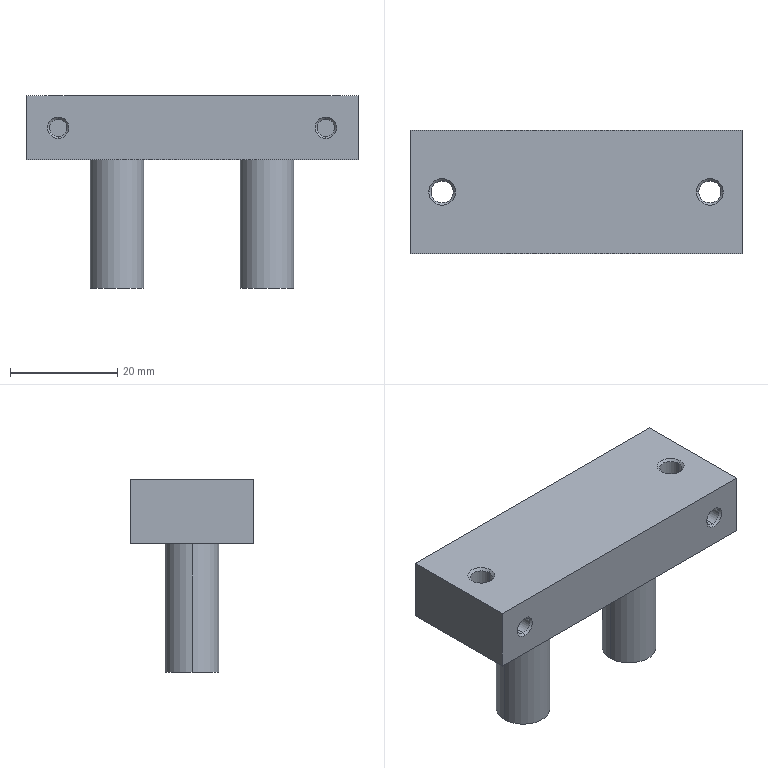Part | STEP file | B_CXSM20-10-Z73 | 1 solid | 40 faces | box 62 x 23 x 36 mm | volume 20357 mm3 | cylinder 16 | cone 12 | plane 12 | commonest cylinder face diameters 3.24 x8 4.13 x4 10 x4
STEP:
#1=CARTESIAN_POINT('',(22.935,12.5,23.565));
#2=VERTEX_POINT('',#1);
#3=CARTESIAN_POINT('',(27.065,12.5,23.565));
#4=VERTEX_POINT('',#3);
#5=CARTESIAN_POINT('',(25.,12.5,23.565));
#6=DIRECTION('',(0.,0.,1.));
#7=DIRECTION('',(1.,0.,0.));
#8=AXIS2_PLACEMENT_3D('',#5,#6,#7);
#9=CIRCLE('',#8,2.065);
#10=EDGE_CURVE('',#2,#4,#9,.T.);
#11=ORIENTED_EDGE('',*,*,#10,.F.);
#12=CARTESIAN_POINT('',(22.5,12.5,24.));
#13=VERTEX_POINT('',#12);
#14=CARTESIAN_POINT('',(22.5,12.5,24.));
#15=DIRECTION('',(-0.7071,0.,0.7071));
#16=VECTOR('',#15,1000.);
#17=LINE('',#14,#16);
#18=EDGE_CURVE('',#2,#13,#17,.T.);
#19=ORIENTED_EDGE('',*,*,#18,.T.);
#20=CARTESIAN_POINT('',(27.5,12.5,24.));
#21=VERTEX_POINT('',#20);
#22=CARTESIAN_POINT('',(25.,12.5,24.));
#23=DIRECTION('',(0.,0.,-1.));
#24=DIRECTION('',(1.,0.,0.));
#25=AXIS2_PLACEMENT_3D('',#22,#23,#24);
#26=CIRCLE('',#25,2.5);
#27=EDGE_CURVE('',#21,#13,#26,.T.);
#28=ORIENTED_EDGE('',*,*,#27,.F.);
#29=CARTESIAN_POINT('',(27.5,12.5,24.));
#30=DIRECTION('',(0.7071,0.,0.7071));
#31=VECTOR('',#30,1000.);
#32=LINE('',#29,#31);
#33=EDGE_CURVE('',#4,#21,#32,.T.);
#34=ORIENTED_EDGE('',*,*,#33,.F.);
#35=EDGE_LOOP('',(#11,#19,#28,#34));
#36=FACE_OUTER_BOUND('',#35,.T.);
#37=CARTESIAN_POINT('',(25.,12.5,24.));
#38=DIRECTION('',(0.,0.,1.));
#39=DIRECTION('',(1.,0.,0.));
#40=AXIS2_PLACEMENT_3D('',#37,#38,#39);
#41=CONICAL_SURFACE('',#40,2.5,0.7854);
#42=ADVANCED_FACE('',(#36),#41,.F.);
#43=CARTESIAN_POINT('',(-27.065,12.5,23.565));
#44=VERTEX_POINT('',#43);
#45=CARTESIAN_POINT('',(-22.935,12.5,23.565));
#46=VERTEX_POINT('',#45);
#47=CARTESIAN_POINT('',(-25.,12.5,23.565));
#48=DIRECTION('',(0.,0.,1.));
#49=DIRECTION('',(1.,0.,0.));
#50=AXIS2_PLACEMENT_3D('',#47,#48,#49);
#51=CIRCLE('',#50,2.065);
#52=EDGE_CURVE('',#44,#46,#51,.T.);
#53=ORIENTED_EDGE('',*,*,#52,.F.);
#54=CARTESIAN_POINT('',(-27.5,12.5,24.));
#55=VERTEX_POINT('',#54);
#56=CARTESIAN_POINT('',(-27.5,12.5,24.));
#57=DIRECTION('',(-0.7071,0.,0.7071));
#58=VECTOR('',#57,1000.);
#59=LINE('',#56,#58);
#60=EDGE_CURVE('',#44,#55,#59,.T.);
#61=ORIENTED_EDGE('',*,*,#60,.T.);
#62=CARTESIAN_POINT('',(-22.5,12.5,24.));
#63=VERTEX_POINT('',#62);
#64=CARTESIAN_POINT('',(-25.,12.5,24.));
#65=DIRECTION('',(0.,0.,-1.));
#66=DIRECTION('',(1.,0.,0.));
#67=AXIS2_PLACEMENT_3D('',#64,#65,#66);
#68=CIRCLE('',#67,2.5);
#69=EDGE_CURVE('',#63,#55,#68,.T.);
#70=ORIENTED_EDGE('',*,*,#69,.F.);
#71=CARTESIAN_POINT('',(-22.5,12.5,24.));
#72=DIRECTION('',(0.7071,0.,0.7071));
#73=VECTOR('',#72,1000.);
#74=LINE('',#71,#73);
#75=EDGE_CURVE('',#46,#63,#74,.T.);
#76=ORIENTED_EDGE('',*,*,#75,.F.);
#77=EDGE_LOOP('',(#53,#61,#70,#76));
#78=FACE_OUTER_BOUND('',#77,.T.);
#79=CARTESIAN_POINT('',(-25.,12.5,24.));
#80=DIRECTION('',(0.,0.,1.));
#81=DIRECTION('',(1.,0.,0.));
#82=AXIS2_PLACEMENT_3D('',#79,#80,#81);
#83=CONICAL_SURFACE('',#82,2.5,0.7854);
#84=ADVANCED_FACE('',(#78),#83,.F.);
#85=CARTESIAN_POINT('',(-25.,23.62,16.38));
#86=VERTEX_POINT('',#85);
#87=CARTESIAN_POINT('',(-25.,23.62,19.62));
#88=VERTEX_POINT('',#87);
#89=CARTESIAN_POINT('',(-25.,23.62,18.));
#90=DIRECTION('',(0.,1.,0.));
#91=DIRECTION('',(-1.,0.,0.));
#92=AXIS2_PLACEMENT_3D('',#89,#90,#91);
#93=CIRCLE('',#92,1.62);
#94=EDGE_CURVE('',#86,#88,#93,.T.);
#95=ORIENTED_EDGE('',*,*,#94,.F.);
#96=CARTESIAN_POINT('',(-25.,24.,16.));
#97=VERTEX_POINT('',#96);
#98=CARTESIAN_POINT('',(-25.,24.,16.));
#99=DIRECTION('',(0.,0.7071,-0.7071));
#100=VECTOR('',#99,1000.);
#101=LINE('',#98,#100);
#102=EDGE_CURVE('',#86,#97,#101,.T.);
#103=ORIENTED_EDGE('',*,*,#102,.T.);
#104=CARTESIAN_POINT('',(-25.,24.,20.));
#105=VERTEX_POINT('',#104);
#106=CARTESIAN_POINT('',(-25.,24.,18.));
#107=DIRECTION('',(0.,-1.,0.));
#108=DIRECTION('',(0.,0.,1.));
#109=AXIS2_PLACEMENT_3D('',#106,#107,#108);
#110=CIRCLE('',#109,2.);
#111=EDGE_CURVE('',#105,#97,#110,.T.);
#112=ORIENTED_EDGE('',*,*,#111,.F.);
#113=CARTESIAN_POINT('',(-25.,24.,20.));
#114=DIRECTION('',(0.,0.7071,0.7071));
#115=VECTOR('',#114,1000.);
#116=LINE('',#113,#115);
#117=EDGE_CURVE('',#88,#105,#116,.T.);
#118=ORIENTED_EDGE('',*,*,#117,.F.);
#119=EDGE_LOOP('',(#95,#103,#112,#118));
#120=FACE_OUTER_BOUND('',#119,.T.);
#121=CARTESIAN_POINT('',(-25.,24.,18.));
#122=DIRECTION('',(0.,1.,0.));
#123=DIRECTION('',(0.,0.,1.));
#124=AXIS2_PLACEMENT_3D('',#121,#122,#123);
#125=CONICAL_SURFACE('',#124,2.,0.7854);
#126=ADVANCED_FACE('',(#120),#125,.F.);
#127=CARTESIAN_POINT('',(25.,23.62,16.38));
#128=VERTEX_POINT('',#127);
#129=CARTESIAN_POINT('',(25.,23.62,19.62));
#130=VERTEX_POINT('',#129);
#131=CARTESIAN_POINT('',(25.,23.62,18.));
#132=DIRECTION('',(0.,1.,0.));
#133=DIRECTION('',(-1.,0.,0.));
#134=AXIS2_PLACEMENT_3D('',#131,#132,#133);
#135=CIRCLE('',#134,1.62);
#136=EDGE_CURVE('',#128,#130,#135,.T.);
#137=ORIENTED_EDGE('',*,*,#136,.F.);
#138=CARTESIAN_POINT('',(25.,24.,16.));
#139=VERTEX_POINT('',#138);
#140=CARTESIAN_POINT('',(25.,24.,16.));
#141=DIRECTION('',(0.,0.7071,-0.7071));
#142=VECTOR('',#141,1000.);
#143=LINE('',#140,#142);
#144=EDGE_CURVE('',#128,#139,#143,.T.);
#145=ORIENTED_EDGE('',*,*,#144,.T.);
#146=CARTESIAN_POINT('',(25.,24.,20.));
#147=VERTEX_POINT('',#146);
#148=CARTESIAN_POINT('',(25.,24.,18.));
#149=DIRECTION('',(0.,-1.,0.));
#150=DIRECTION('',(0.,0.,1.));
#151=AXIS2_PLACEMENT_3D('',#148,#149,#150);
#152=CIRCLE('',#151,2.);
#153=EDGE_CURVE('',#147,#139,#152,.T.);
#154=ORIENTED_EDGE('',*,*,#153,.F.);
#155=CARTESIAN_POINT('',(25.,24.,20.));
#156=DIRECTION('',(0.,0.7071,0.7071));
#157=VECTOR('',#156,1000.);
#158=LINE('',#155,#157);
#159=EDGE_CURVE('',#130,#147,#158,.T.);
#160=ORIENTED_EDGE('',*,*,#159,.F.);
#161=EDGE_LOOP('',(#137,#145,#154,#160));
#162=FACE_OUTER_BOUND('',#161,.T.);
#163=CARTESIAN_POINT('',(25.,24.,18.));
#164=DIRECTION('',(0.,1.,0.));
#165=DIRECTION('',(0.,0.,1.));
#166=AXIS2_PLACEMENT_3D('',#163,#164,#165);
#167=CONICAL_SURFACE('',#166,2.,0.7854);
#168=ADVANCED_FACE('',(#162),#167,.F.);
#169=CARTESIAN_POINT('',(25.,1.38,19.62));
#170=VERTEX_POINT('',#169);
#171=CARTESIAN_POINT('',(25.,1.38,16.38));
#172=VERTEX_POINT('',#171);
#173=CARTESIAN_POINT('',(25.,1.38,18.));
#174=DIRECTION('',(0.,-1.,0.));
#175=DIRECTION('',(1.,0.,0.));
#176=AXIS2_PLACEMENT_3D('',#173,#174,#175);
#177=CIRCLE('',#176,1.62);
#178=EDGE_CURVE('',#170,#172,#177,.T.);
#179=ORIENTED_EDGE('',*,*,#178,.F.);
#180=CARTESIAN_POINT('',(25.,1.,20.));
#181=VERTEX_POINT('',#180);
#182=CARTESIAN_POINT('',(25.,1.,20.));
#183=DIRECTION('',(0.,-0.7071,0.7071));
#184=VECTOR('',#183,1000.);
#185=LINE('',#182,#184);
#186=EDGE_CURVE('',#170,#181,#185,.T.);
#187=ORIENTED_EDGE('',*,*,#186,.T.);
#188=CARTESIAN_POINT('',(25.,1.,16.));
#189=VERTEX_POINT('',#188);
#190=CARTESIAN_POINT('',(25.,1.,18.));
#191=DIRECTION('',(0.,1.,0.));
#192=DIRECTION('',(0.,0.,-1.));
#193=AXIS2_PLACEMENT_3D('',#190,#191,#192);
#194=CIRCLE('',#193,2.);
#195=EDGE_CURVE('',#189,#181,#194,.T.);
#196=ORIENTED_EDGE('',*,*,#195,.F.);
#197=CARTESIAN_POINT('',(25.,1.,16.));
#198=DIRECTION('',(0.,-0.7071,-0.7071));
#199=VECTOR('',#198,1000.);
#200=LINE('',#197,#199);
#201=EDGE_CURVE('',#172,#189,#200,.T.);
#202=ORIENTED_EDGE('',*,*,#201,.F.);
#203=EDGE_LOOP('',(#179,#187,#196,#202));
#204=FACE_OUTER_BOUND('',#203,.T.);
#205=CARTESIAN_POINT('',(25.,1.,18.));
#206=DIRECTION('',(0.,-1.,0.));
#207=DIRECTION('',(0.,0.,-1.));
#208=AXIS2_PLACEMENT_3D('',#205,#206,#207);
#209=CONICAL_SURFACE('',#208,2.,0.7854);
#210=ADVANCED_FACE('',(#204),#209,.F.);
#211=CARTESIAN_POINT('',(-25.,1.38,19.62));
#212=VERTEX_POINT('',#211);
#213=CARTESIAN_POINT('',(-25.,1.38,16.38));
#214=VERTEX_POINT('',#213);
#215=CARTESIAN_POINT('',(-25.,1.38,18.));
#216=DIRECTION('',(0.,-1.,0.));
#217=DIRECTION('',(1.,0.,0.));
#218=AXIS2_PLACEMENT_3D('',#215,#216,#217);
#219=CIRCLE('',#218,1.62);
#220=EDGE_CURVE('',#212,#214,#219,.T.);
#221=ORIENTED_EDGE('',*,*,#220,.F.);
#222=CARTESIAN_POINT('',(-25.,1.,20.));
#223=VERTEX_POINT('',#222);
#224=CARTESIAN_POINT('',(-25.,1.,20.));
#225=DIRECTION('',(0.,-0.7071,0.7071));
#226=VECTOR('',#225,1000.);
#227=LINE('',#224,#226);
#228=EDGE_CURVE('',#212,#223,#227,.T.);
#229=ORIENTED_EDGE('',*,*,#228,.T.);
#230=CARTESIAN_POINT('',(-25.,1.,16.));
#231=VERTEX_POINT('',#230);
#232=CARTESIAN_POINT('',(-25.,1.,18.));
#233=DIRECTION('',(0.,1.,0.));
#234=DIRECTION('',(0.,0.,-1.));
#235=AXIS2_PLACEMENT_3D('',#232,#233,#234);
#236=CIRCLE('',#235,2.);
#237=EDGE_CURVE('',#231,#223,#236,.T.);
#238=ORIENTED_EDGE('',*,*,#237,.F.);
#239=CARTESIAN_POINT('',(-25.,1.,16.));
#240=DIRECTION('',(0.,-0.7071,-0.7071));
#241=VECTOR('',#240,1000.);
#242=LINE('',#239,#241);
#243=EDGE_CURVE('',#214,#231,#242,.T.);
#244=ORIENTED_EDGE('',*,*,#243,.F.);
#245=EDGE_LOOP('',(#221,#229,#238,#244));
#246=FACE_OUTER_BOUND('',#245,.T.);
#247=CARTESIAN_POINT('',(-25.,1.,18.));
#248=DIRECTION('',(0.,-1.,0.));
#249=DIRECTION('',(0.,0.,-1.));
#250=AXIS2_PLACEMENT_3D('',#247,#248,#249);
#251=CONICAL_SURFACE('',#250,2.,0.7854);
#252=ADVANCED_FACE('',(#246),#251,.F.);
#253=CARTESIAN_POINT('',(27.065,12.5,12.));
#254=VERTEX_POINT('',#253);
#255=CARTESIAN_POINT('',(22.935,12.5,12.));
#256=VERTEX_POINT('',#255);
#257=CARTESIAN_POINT('',(25.,12.5,12.));
#258=DIRECTION('',(0.,0.,-1.));
#259=DIRECTION('',(1.,0.,0.));
#260=AXIS2_PLACEMENT_3D('',#257,#258,#259);
#261=CIRCLE('',#260,2.065);
#262=EDGE_CURVE('',#254,#256,#261,.T.);
#263=ORIENTED_EDGE('',*,*,#262,.T.);
#264=CARTESIAN_POINT('',(22.935,12.5,17.782));
#265=DIRECTION('',(0.,0.,1.));
#266=VECTOR('',#265,1000.);
#267=LINE('',#264,#266);
#268=EDGE_CURVE('',#256,#2,#267,.T.);
#269=ORIENTED_EDGE('',*,*,#268,.T.);
#270=ORIENTED_EDGE('',*,*,#10,.T.);
#271=CARTESIAN_POINT('',(27.065,12.5,17.782));
#272=DIRECTION('',(0.,0.,1.));
#273=VECTOR('',#272,1000.);
#274=LINE('',#271,#273);
#275=EDGE_CURVE('',#254,#4,#274,.T.);
#276=ORIENTED_EDGE('',*,*,#275,.F.);
#277=EDGE_LOOP('',(#263,#269,#270,#276));
#278=FACE_OUTER_BOUND('',#277,.T.);
#279=CARTESIAN_POINT('',(25.,12.5,17.782));
#280=DIRECTION('',(0.,0.,1.));
#281=DIRECTION('',(1.,0.,0.));
#282=AXIS2_PLACEMENT_3D('',#279,#280,#281);
#283=CYLINDRICAL_SURFACE('',#282,2.065);
#284=ADVANCED_FACE('',(#278),#283,.F.);
#285=CARTESIAN_POINT('',(-22.935,12.5,12.));
#286=VERTEX_POINT('',#285);
#287=CARTESIAN_POINT('',(-27.065,12.5,12.));
#288=VERTEX_POINT('',#287);
#289=CARTESIAN_POINT('',(-25.,12.5,12.));
#290=DIRECTION('',(0.,0.,-1.));
#291=DIRECTION('',(1.,0.,0.));
#292=AXIS2_PLACEMENT_3D('',#289,#290,#291);
#293=CIRCLE('',#292,2.065);
#294=EDGE_CURVE('',#286,#288,#293,.T.);
#295=ORIENTED_EDGE('',*,*,#294,.T.);
#296=CARTESIAN_POINT('',(-27.065,12.5,17.782));
#297=DIRECTION('',(0.,0.,1.));
#298=VECTOR('',#297,1000.);
#299=LINE('',#296,#298);
#300=EDGE_CURVE('',#288,#44,#299,.T.);
#301=ORIENTED_EDGE('',*,*,#300,.T.);
#302=ORIENTED_EDGE('',*,*,#52,.T.);
#303=CARTESIAN_POINT('',(-22.935,12.5,17.782));
#304=DIRECTION('',(0.,0.,1.));
#305=VECTOR('',#304,1000.);
#306=LINE('',#303,#305);
#307=EDGE_CURVE('',#286,#46,#306,.T.);
#308=ORIENTED_EDGE('',*,*,#307,.F.);
#309=EDGE_LOOP('',(#295,#301,#302,#308));
#310=FACE_OUTER_BOUND('',#309,.T.);
#311=CARTESIAN_POINT('',(-25.,12.5,17.782));
#312=DIRECTION('',(0.,0.,1.));
#313=DIRECTION('',(1.,0.,0.));
#314=AXIS2_PLACEMENT_3D('',#311,#312,#313);
#315=CYLINDRICAL_SURFACE('',#314,2.065);
#316=ADVANCED_FACE('',(#310),#315,.F.);
#317=CARTESIAN_POINT('',(19.,12.5,-12.));
#318=VERTEX_POINT('',#317);
#319=CARTESIAN_POINT('',(9.,12.5,-12.));
#320=VERTEX_POINT('',#319);
#321=CARTESIAN_POINT('',(14.,12.5,-12.));
#322=DIRECTION('',(0.,0.,1.));
#323=DIRECTION('',(1.,0.,0.));
#324=AXIS2_PLACEMENT_3D('',#321,#322,#323);
#325=CIRCLE('',#324,5.);
#326=EDGE_CURVE('',#318,#320,#325,.T.);
#327=ORIENTED_EDGE('',*,*,#326,.T.);
#328=CARTESIAN_POINT('',(9.,12.5,12.));
#329=VERTEX_POINT('',#328);
#330=CARTESIAN_POINT('',(9.,12.5,12.));
#331=DIRECTION('',(0.,0.,1.));
#332=VECTOR('',#331,1000.);
#333=LINE('',#330,#332);
#334=EDGE_CURVE('',#320,#329,#333,.T.);
#335=ORIENTED_EDGE('',*,*,#334,.T.);
#336=CARTESIAN_POINT('',(19.,12.5,12.));
#337=VERTEX_POINT('',#336);
#338=CARTESIAN_POINT('',(14.,12.5,12.));
#339=DIRECTION('',(0.,0.,-1.));
#340=DIRECTION('',(1.,0.,0.));
#341=AXIS2_PLACEMENT_3D('',#338,#339,#340);
#342=CIRCLE('',#341,5.);
#343=EDGE_CURVE('',#329,#337,#342,.T.);
#344=ORIENTED_EDGE('',*,*,#343,.T.);
#345=CARTESIAN_POINT('',(19.,12.5,12.));
#346=DIRECTION('',(0.,0.,1.));
#347=VECTOR('',#346,1000.);
#348=LINE('',#345,#347);
#349=EDGE_CURVE('',#318,#337,#348,.T.);
#350=ORIENTED_EDGE('',*,*,#349,.F.);
#351=EDGE_LOOP('',(#327,#335,#344,#350));
#352=FACE_OUTER_BOUND('',#351,.T.);
#353=CARTESIAN_POINT('',(14.,12.5,12.));
#354=DIRECTION('',(0.,0.,1.));
#355=DIRECTION('',(1.,0.,0.));
#356=AXIS2_PLACEMENT_3D('',#353,#354,#355);
#357=CYLINDRICAL_SURFACE('',#356,5.);
#358=ADVANCED_FACE('',(#352),#357,.T.);
#359=CARTESIAN_POINT('',(-9.,12.5,-12.));
#360=VERTEX_POINT('',#359);
#361=CARTESIAN_POINT('',(-19.,12.5,-12.));
#362=VERTEX_POINT('',#361);
#363=CARTESIAN_POINT('',(-14.,12.5,-12.));
#364=DIRECTION('',(0.,0.,1.));
#365=DIRECTION('',(1.,0.,0.));
#366=AXIS2_PLACEMENT_3D('',#363,#364,#365);
#367=CIRCLE('',#366,5.);
#368=EDGE_CURVE('',#360,#362,#367,.T.);
#369=ORIENTED_EDGE('',*,*,#368,.T.);
#370=CARTESIAN_POINT('',(-19.,12.5,12.));
#371=VERTEX_POINT('',#370);
#372=CARTESIAN_POINT('',(-19.,12.5,12.));
#373=DIRECTION('',(0.,0.,1.));
#374=VECTOR('',#373,1000.);
#375=LINE('',#372,#374);
#376=EDGE_CURVE('',#362,#371,#375,.T.);
#377=ORIENTED_EDGE('',*,*,#376,.T.);
#378=CARTESIAN_POINT('',(-9.,12.5,12.));
#379=VERTEX_POINT('',#378);
#380=CARTESIAN_POINT('',(-14.,12.5,12.));
#381=DIRECTION('',(0.,0.,-1.));
#382=DIRECTION('',(1.,0.,0.));
#383=AXIS2_PLACEMENT_3D('',#380,#381,#382);
#384=CIRCLE('',#383,5.);
#385=EDGE_CURVE('',#371,#379,#384,.T.);
#386=ORIENTED_EDGE('',*,*,#385,.T.);
#387=CARTESIAN_POINT('',(-9.,12.5,12.));
#388=DIRECTION('',(0.,0.,1.));
#389=VECTOR('',#388,1000.);
#390=LINE('',#387,#389);
#391=EDGE_CURVE('',#360,#379,#390,.T.);
#392=ORIENTED_EDGE('',*,*,#391,.F.);
#393=EDGE_LOOP('',(#369,#377,#386,#392));
#394=FACE_OUTER_BOUND('',#393,.T.);
#395=CARTESIAN_POINT('',(-14.,12.5,12.));
#396=DIRECTION('',(0.,0.,1.));
#397=DIRECTION('',(1.,0.,0.));
#398=AXIS2_PLACEMENT_3D('',#395,#396,#397);
#399=CYLINDRICAL_SURFACE('',#398,5.);
#400=ADVANCED_FACE('',(#394),#399,.T.);
#401=CARTESIAN_POINT('',(-25.,18.,16.38));
#402=VERTEX_POINT('',#401);
#403=CARTESIAN_POINT('',(-25.,18.,19.62));
#404=VERTEX_POINT('',#403);
#405=CARTESIAN_POINT('',(-25.,18.,18.));
#406=DIRECTION('',(0.,1.,0.));
#407=DIRECTION('',(0.,0.,1.));
#408=AXIS2_PLACEMENT_3D('',#405,#406,#407);
#409=CIRCLE('',#408,1.62);
#410=EDGE_CURVE('',#402,#404,#409,.T.);
#411=ORIENTED_EDGE('',*,*,#410,.F.);
#412=CARTESIAN_POINT('',(-25.,20.81,16.38));
#413=DIRECTION('',(0.,1.,0.));
#414=VECTOR('',#413,1000.);
#415=LINE('',#412,#414);
#416=EDGE_CURVE('',#402,#86,#415,.T.);
#417=ORIENTED_EDGE('',*,*,#416,.T.);
#418=ORIENTED_EDGE('',*,*,#94,.T.);
#419=CARTESIAN_POINT('',(-25.,20.81,19.62));
#420=DIRECTION('',(0.,1.,0.));
#421=VECTOR('',#420,1000.);
#422=LINE('',#419,#421);
#423=EDGE_CURVE('',#404,#88,#422,.T.);
#424=ORIENTED_EDGE('',*,*,#423,.F.);
#425=EDGE_LOOP('',(#411,#417,#418,#424));
#426=FACE_OUTER_BOUND('',#425,.T.);
#427=CARTESIAN_POINT('',(-25.,20.81,18.));
#428=DIRECTION('',(0.,1.,0.));
#429=DIRECTION('',(0.,0.,1.));
#430=AXIS2_PLACEMENT_3D('',#427,#428,#429);
#431=CYLINDRICAL_SURFACE('',#430,1.62);
#432=ADVANCED_FACE('',(#426),#431,.F.);
#433=CARTESIAN_POINT('',(25.,18.,16.38));
#434=VERTEX_POINT('',#433);
#435=CARTESIAN_POINT('',(25.,18.,19.62));
#436=VERTEX_POINT('',#435);
#437=CARTESIAN_POINT('',(25.,18.,18.));
#438=DIRECTION('',(0.,1.,0.));
#439=DIRECTION('',(0.,0.,1.));
#440=AXIS2_PLACEMENT_3D('',#437,#438,#439);
#441=CIRCLE('',#440,1.62);
#442=EDGE_CURVE('',#434,#436,#441,.T.);
#443=ORIENTED_EDGE('',*,*,#442,.F.);
#444=CARTESIAN_POINT('',(25.,20.81,16.38));
#445=DIRECTION('',(0.,1.,0.));
#446=VECTOR('',#445,1000.);
#447=LINE('',#444,#446);
#448=EDGE_CURVE('',#434,#128,#447,.T.);
#449=ORIENTED_EDGE('',*,*,#448,.T.);
#450=ORIENTED_EDGE('',*,*,#136,.T.);
#451=CARTESIAN_POINT('',(25.,20.81,19.62));
#452=DIRECTION('',(0.,1.,0.));
#453=VECTOR('',#452,1000.);
#454=LINE('',#451,#453);
#455=EDGE_CURVE('',#436,#130,#454,.T.);
#456=ORIENTED_EDGE('',*,*,#455,.F.);
#457=EDGE_LOOP('',(#443,#449,#450,#456));
#458=FACE_OUTER_BOUND('',#457,.T.);
#459=CARTESIAN_POINT('',(25.,20.81,18.));
#460=DIRECTION('',(0.,1.,0.));
#461=DIRECTION('',(0.,0.,1.));
#462=AXIS2_PLACEMENT_3D('',#459,#460,#461);
#463=CYLINDRICAL_SURFACE('',#462,1.62);
#464=ADVANCED_FACE('',(#458),#463,.F.);
#465=CARTESIAN_POINT('',(25.,7.,19.62));
#466=VERTEX_POINT('',#465);
#467=CARTESIAN_POINT('',(25.,7.,16.38));
#468=VERTEX_POINT('',#467);
#469=CARTESIAN_POINT('',(25.,7.,18.));
#470=DIRECTION('',(0.,-1.,0.));
#471=DIRECTION('',(0.,0.,-1.));
#472=AXIS2_PLACEMENT_3D('',#469,#470,#471);
#473=CIRCLE('',#472,1.62);
#474=EDGE_CURVE('',#466,#468,#473,.T.);
#475=ORIENTED_EDGE('',*,*,#474,.F.);
#476=CARTESIAN_POINT('',(25.,4.19,19.62));
#477=DIRECTION('',(0.,-1.,0.));
#478=VECTOR('',#477,1000.);
#479=LINE('',#476,#478);
#480=EDGE_CURVE('',#466,#170,#479,.T.);
#481=ORIENTED_EDGE('',*,*,#480,.T.);
#482=ORIENTED_EDGE('',*,*,#178,.T.);
#483=CARTESIAN_POINT('',(25.,4.19,16.38));
#484=DIRECTION('',(0.,-1.,0.));
#485=VECTOR('',#484,1000.);
#486=LINE('',#483,#485);
#487=EDGE_CURVE('',#468,#172,#486,.T.);
#488=ORIENTED_EDGE('',*,*,#487,.F.);
#489=EDGE_LOOP('',(#475,#481,#482,#488));
#490=FACE_OUTER_BOUND('',#489,.T.);
#491=CARTESIAN_POINT('',(25.,4.19,18.));
#492=DIRECTION('',(0.,-1.,0.));
#493=DIRECTION('',(0.,0.,-1.));
#494=AXIS2_PLACEMENT_3D('',#491,#492,#493);
#495=CYLINDRICAL_SURFACE('',#494,1.62);
#496=ADVANCED_FACE('',(#490),#495,.F.);
#497=CARTESIAN_POINT('',(-25.,7.,19.62));
#498=VERTEX_POINT('',#497);
#499=CARTESIAN_POINT('',(-25.,7.,16.38));
#500=VERTEX_POINT('',#499);
#501=CARTESIAN_POINT('',(-25.,7.,18.));
#502=DIRECTION('',(0.,-1.,0.));
#503=DIRECTION('',(0.,0.,-1.));
#504=AXIS2_PLACEMENT_3D('',#501,#502,#503);
#505=CIRCLE('',#504,1.62);
#506=EDGE_CURVE('',#498,#500,#505,.T.);
#507=ORIENTED_EDGE('',*,*,#506,.F.);
#508=CARTESIAN_POINT('',(-25.,4.19,19.62));
#509=DIRECTION('',(0.,-1.,0.));
#510=VECTOR('',#509,1000.);
#511=LINE('',#508,#510);
#512=EDGE_CURVE('',#498,#212,#511,.T.);
#513=ORIENTED_EDGE('',*,*,#512,.T.);
#514=ORIENTED_EDGE('',*,*,#220,.T.);
#515=CARTESIAN_POINT('',(-25.,4.19,16.38));
#516=DIRECTION('',(0.,-1.,0.));
#517=VECTOR('',#516,1000.);
#518=LINE('',#515,#517);
#519=EDGE_CURVE('',#500,#214,#518,.T.);
#520=ORIENTED_EDGE('',*,*,#519,.F.);
#521=EDGE_LOOP('',(#507,#513,#514,#520));
#522=FACE_OUTER_BOUND('',#521,.T.);
#523=CARTESIAN_POINT('',(-25.,4.19,18.));
#524=DIRECTION('',(0.,-1.,0.));
#525=DIRECTION('',(0.,0.,-1.));
#526=AXIS2_PLACEMENT_3D('',#523,#524,#525);
#527=CYLINDRICAL_SURFACE('',#526,1.62);
#528=ADVANCED_FACE('',(#522),#527,.F.);
#529=CARTESIAN_POINT('',(31.,1.,24.));
#530=VERTEX_POINT('',#529);
#531=CARTESIAN_POINT('',(31.,24.,24.));
#532=VERTEX_POINT('',#531);
#533=CARTESIAN_POINT('',(31.,0.,24.));
#534=DIRECTION('',(0.,1.,0.));
#535=VECTOR('',#534,1000.);
#536=LINE('',#533,#535);
#537=EDGE_CURVE('',#530,#532,#536,.T.);
#538=ORIENTED_EDGE('',*,*,#537,.T.);
#539=CARTESIAN_POINT('',(-31.,24.,24.));
#540=VERTEX_POINT('',#539);
#541=CARTESIAN_POINT('',(0.,24.,24.));
#542=DIRECTION('',(-1.,0.,0.));
#543=VECTOR('',#542,1000.);
#544=LINE('',#541,#543);
#545=EDGE_CURVE('',#532,#540,#544,.T.);
#546=ORIENTED_EDGE('',*,*,#545,.T.);
#547=CARTESIAN_POINT('',(-31.,1.,24.));
#548=VERTEX_POINT('',#547);
#549=CARTESIAN_POINT('',(-31.,0.,24.));
#550=DIRECTION('',(0.,-1.,0.));
#551=VECTOR('',#550,1000.);
#552=LINE('',#549,#551);
#553=EDGE_CURVE('',#540,#548,#552,.T.);
#554=ORIENTED_EDGE('',*,*,#553,.T.);
#555=CARTESIAN_POINT('',(0.,1.,24.));
#556=DIRECTION('',(1.,0.,0.));
#557=VECTOR('',#556,1000.);
#558=LINE('',#555,#557);
#559=EDGE_CURVE('',#548,#530,#558,.T.);
#560=ORIENTED_EDGE('',*,*,#559,.T.);
#561=EDGE_LOOP('',(#538,#546,#554,#560));
#562=FACE_OUTER_BOUND('',#561,.T.);
#563=ORIENTED_EDGE('',*,*,#27,.T.);
#564=CARTESIAN_POINT('',(25.,12.5,24.));
#565=DIRECTION('',(0.,0.,-1.));
#566=DIRECTION('',(1.,0.,0.));
#567=AXIS2_PLACEMENT_3D('',#564,#565,#566);
#568=CIRCLE('',#567,2.5);
#569=EDGE_CURVE('',#13,#21,#568,.T.);
#570=ORIENTED_EDGE('',*,*,#569,.T.);
#571=EDGE_LOOP('',(#563,#570));
#572=FACE_BOUND('',#571,.T.);
#573=ORIENTED_EDGE('',*,*,#69,.T.);
#574=CARTESIAN_POINT('',(-25.,12.5,24.));
#575=DIRECTION('',(0.,0.,-1.));
#576=DIRECTION('',(1.,0.,0.));
#577=AXIS2_PLACEMENT_3D('',#574,#575,#576);
#578=CIRCLE('',#577,2.5);
#579=EDGE_CURVE('',#55,#63,#578,.T.);
#580=ORIENTED_EDGE('',*,*,#579,.T.);
#581=EDGE_LOOP('',(#573,#580));
#582=FACE_BOUND('',#581,.T.);
#583=CARTESIAN_POINT('',(0.,0.,24.));
#584=DIRECTION('',(0.,0.,1.));
#585=DIRECTION('',(1.,0.,0.));
#586=AXIS2_PLACEMENT_3D('',#583,#584,#585);
#587=PLANE('',#586);
#588=ADVANCED_FACE('',(#562,#572,#582),#587,.T.);
#589=CARTESIAN_POINT('',(31.,24.,12.));
#590=VERTEX_POINT('',#589);
#591=CARTESIAN_POINT('',(-31.,24.,12.));
#592=VERTEX_POINT('',#591);
#593=CARTESIAN_POINT('',(-31.,24.,12.));
#594=DIRECTION('',(-1.,0.,0.));
#595=VECTOR('',#594,1000.);
#596=LINE('',#593,#595);
#597=EDGE_CURVE('',#590,#592,#596,.T.);
#598=ORIENTED_EDGE('',*,*,#597,.T.);
#599=CARTESIAN_POINT('',(-31.,24.,12.));
#600=DIRECTION('',(0.,0.,1.));
#601=VECTOR('',#600,1000.);
#602=LINE('',#599,#601);
#603=EDGE_CURVE('',#592,#540,#602,.T.);
#604=ORIENTED_EDGE('',*,*,#603,.T.);
#605=ORIENTED_EDGE('',*,*,#545,.F.);
#606=CARTESIAN_POINT('',(31.,24.,12.));
#607=DIRECTION('',(0.,0.,-1.));
#608=VECTOR('',#607,1000.);
#609=LINE('',#606,#608);
#610=EDGE_CURVE('',#532,#590,#609,.T.);
#611=ORIENTED_EDGE('',*,*,#610,.T.);
#612=EDGE_LOOP('',(#598,#604,#605,#611));
#613=FACE_OUTER_BOUND('',#612,.T.);
#614=ORIENTED_EDGE('',*,*,#111,.T.);
#615=CARTESIAN_POINT('',(-25.,24.,18.));
#616=DIRECTION('',(0.,-1.,0.));
#617=DIRECTION('',(0.,0.,1.));
#618=AXIS2_PLACEMENT_3D('',#615,#616,#617);
#619=CIRCLE('',#618,2.);
#620=EDGE_CURVE('',#97,#105,#619,.T.);
#621=ORIENTED_EDGE('',*,*,#620,.T.);
#622=EDGE_LOOP('',(#614,#621));
#623=FACE_BOUND('',#622,.T.);
#624=ORIENTED_EDGE('',*,*,#153,.T.);
#625=CARTESIAN_POINT('',(25.,24.,18.));
#626=DIRECTION('',(0.,-1.,0.));
#627=DIRECTION('',(0.,0.,1.));
#628=AXIS2_PLACEMENT_3D('',#625,#626,#627);
#629=CIRCLE('',#628,2.);
#630=EDGE_CURVE('',#139,#147,#629,.T.);
#631=ORIENTED_EDGE('',*,*,#630,.T.);
#632=EDGE_LOOP('',(#624,#631));
#633=FACE_BOUND('',#632,.T.);
#634=CARTESIAN_POINT('',(-31.,24.,12.));
#635=DIRECTION('',(0.,1.,0.));
#636=DIRECTION('',(0.,0.,1.));
#637=AXIS2_PLACEMENT_3D('',#634,#635,#636);
#638=PLANE('',#637);
#639=ADVANCED_FACE('',(#613,#623,#633),#638,.T.);
#640=CARTESIAN_POINT('',(31.,1.,12.));
#641=VERTEX_POINT('',#640);
#642=CARTESIAN_POINT('',(31.,24.,12.));
#643=DIRECTION('',(0.,1.,0.));
#644=VECTOR('',#643,1000.);
#645=LINE('',#642,#644);
#646=EDGE_CURVE('',#641,#590,#645,.T.);
#647=ORIENTED_EDGE('',*,*,#646,.T.);
#648=ORIENTED_EDGE('',*,*,#610,.F.);
#649=ORIENTED_EDGE('',*,*,#537,.F.);
#650=CARTESIAN_POINT('',(31.,1.,12.));
#651=DIRECTION('',(0.,0.,-1.));
#652=VECTOR('',#651,1000.);
#653=LINE('',#650,#652);
#654=EDGE_CURVE('',#530,#641,#653,.T.);
#655=ORIENTED_EDGE('',*,*,#654,.T.);
#656=EDGE_LOOP('',(#647,#648,#649,#655));
#657=FACE_OUTER_BOUND('',#656,.T.);
#658=CARTESIAN_POINT('',(31.,24.,12.));
#659=DIRECTION('',(1.,0.,0.));
#660=DIRECTION('',(0.,0.,-1.));
#661=AXIS2_PLACEMENT_3D('',#658,#659,#660);
#662=PLANE('',#661);
#663=ADVANCED_FACE('',(#657),#662,.T.);
#664=CARTESIAN_POINT('',(-31.,1.,12.));
#665=VERTEX_POINT('',#664);
#666=CARTESIAN_POINT('',(31.,1.,12.));
#667=DIRECTION('',(1.,0.,0.));
#668=VECTOR('',#667,1000.);
#669=LINE('',#666,#668);
#670=EDGE_CURVE('',#665,#641,#669,.T.);
#671=ORIENTED_EDGE('',*,*,#670,.T.);
#672=ORIENTED_EDGE('',*,*,#654,.F.);
#673=ORIENTED_EDGE('',*,*,#559,.F.);
#674=CARTESIAN_POINT('',(-31.,1.,12.));
#675=DIRECTION('',(0.,0.,-1.));
#676=VECTOR('',#675,1000.);
#677=LINE('',#674,#676);
#678=EDGE_CURVE('',#548,#665,#677,.T.);
#679=ORIENTED_EDGE('',*,*,#678,.T.);
#680=EDGE_LOOP('',(#671,#672,#673,#679));
#681=FACE_OUTER_BOUND('',#680,.T.);
#682=ORIENTED_EDGE('',*,*,#195,.T.);
#683=CARTESIAN_POINT('',(25.,1.,18.));
#684=DIRECTION('',(0.,1.,0.));
#685=DIRECTION('',(0.,0.,-1.));
#686=AXIS2_PLACEMENT_3D('',#683,#684,#685);
#687=CIRCLE('',#686,2.);
#688=EDGE_CURVE('',#181,#189,#687,.T.);
#689=ORIENTED_EDGE('',*,*,#688,.T.);
#690=EDGE_LOOP('',(#682,#689));
#691=FACE_BOUND('',#690,.T.);
#692=ORIENTED_EDGE('',*,*,#237,.T.);
#693=CARTESIAN_POINT('',(-25.,1.,18.));
#694=DIRECTION('',(0.,1.,0.));
#695=DIRECTION('',(0.,0.,-1.));
#696=AXIS2_PLACEMENT_3D('',#693,#694,#695);
#697=CIRCLE('',#696,2.);
#698=EDGE_CURVE('',#223,#231,#697,.T.);
#699=ORIENTED_EDGE('',*,*,#698,.T.);
#700=EDGE_LOOP('',(#692,#699));
#701=FACE_BOUND('',#700,.T.);
#702=CARTESIAN_POINT('',(31.,1.,12.));
#703=DIRECTION('',(0.,-1.,0.));
#704=DIRECTION('',(0.,0.,-1.));
#705=AXIS2_PLACEMENT_3D('',#702,#703,#704);
#706=PLANE('',#705);
#707=ADVANCED_FACE('',(#681,#691,#701),#706,.T.);
#708=CARTESIAN_POINT('',(-31.,1.,12.));
#709=DIRECTION('',(0.,-1.,0.));
#710=VECTOR('',#709,1000.);
#711=LINE('',#708,#710);
#712=EDGE_CURVE('',#592,#665,#711,.T.);
#713=ORIENTED_EDGE('',*,*,#712,.T.);
#714=ORIENTED_EDGE('',*,*,#678,.F.);
#715=ORIENTED_EDGE('',*,*,#553,.F.);
#716=ORIENTED_EDGE('',*,*,#603,.F.);
#717=EDGE_LOOP('',(#713,#714,#715,#716));
#718=FACE_OUTER_BOUND('',#717,.T.);
#719=CARTESIAN_POINT('',(-31.,1.,12.));
#720=DIRECTION('',(-1.,0.,0.));
#721=DIRECTION('',(0.,0.,1.));
#722=AXIS2_PLACEMENT_3D('',#719,#720,#721);
#723=PLANE('',#722);
#724=ADVANCED_FACE('',(#718),#723,.T.);
#725=ORIENTED_EDGE('',*,*,#18,.F.);
#726=CARTESIAN_POINT('',(25.,12.5,23.565));
#727=DIRECTION('',(0.,0.,1.));
#728=DIRECTION('',(1.,0.,0.));
#729=AXIS2_PLACEMENT_3D('',#726,#727,#728);
#730=CIRCLE('',#729,2.065);
#731=EDGE_CURVE('',#4,#2,#730,.T.);
#732=ORIENTED_EDGE('',*,*,#731,.F.);
#733=ORIENTED_EDGE('',*,*,#33,.T.);
#734=ORIENTED_EDGE('',*,*,#569,.F.);
#735=EDGE_LOOP('',(#725,#732,#733,#734));
#736=FACE_OUTER_BOUND('',#735,.T.);
#737=CARTESIAN_POINT('',(25.,12.5,24.));
#738=DIRECTION('',(0.,0.,1.));
#739=DIRECTION('',(1.,0.,0.));
#740=AXIS2_PLACEMENT_3D('',#737,#738,#739);
#741=CONICAL_SURFACE('',#740,2.5,0.7854);
#742=ADVANCED_FACE('',(#736),#741,.F.);
#743=ORIENTED_EDGE('',*,*,#60,.F.);
#744=CARTESIAN_POINT('',(-25.,12.5,23.565));
#745=DIRECTION('',(0.,0.,1.));
#746=DIRECTION('',(1.,0.,0.));
#747=AXIS2_PLACEMENT_3D('',#744,#745,#746);
#748=CIRCLE('',#747,2.065);
#749=EDGE_CURVE('',#46,#44,#748,.T.);
#750=ORIENTED_EDGE('',*,*,#749,.F.);
#751=ORIENTED_EDGE('',*,*,#75,.T.);
#752=ORIENTED_EDGE('',*,*,#579,.F.);
#753=EDGE_LOOP('',(#743,#750,#751,#752));
#754=FACE_OUTER_BOUND('',#753,.T.);
#755=CARTESIAN_POINT('',(-25.,12.5,24.));
#756=DIRECTION('',(0.,0.,1.));
#757=DIRECTION('',(1.,0.,0.));
#758=AXIS2_PLACEMENT_3D('',#755,#756,#757);
#759=CONICAL_SURFACE('',#758,2.5,0.7854);
#760=ADVANCED_FACE('',(#754),#759,.F.);
#761=ORIENTED_EDGE('',*,*,#712,.F.);
#762=ORIENTED_EDGE('',*,*,#597,.F.);
#763=ORIENTED_EDGE('',*,*,#646,.F.);
#764=ORIENTED_EDGE('',*,*,#670,.F.);
#765=EDGE_LOOP('',(#761,#762,#763,#764));
#766=FACE_OUTER_BOUND('',#765,.T.);
#767=CARTESIAN_POINT('',(14.,12.5,12.));
#768=DIRECTION('',(0.,0.,-1.));
#769=DIRECTION('',(1.,0.,0.));
#770=AXIS2_PLACEMENT_3D('',#767,#768,#769);
#771=CIRCLE('',#770,5.);
#772=EDGE_CURVE('',#337,#329,#771,.T.);
#773=ORIENTED_EDGE('',*,*,#772,.F.);
#774=ORIENTED_EDGE('',*,*,#343,.F.);
#775=EDGE_LOOP('',(#773,#774));
#776=FACE_BOUND('',#775,.T.);
#777=CARTESIAN_POINT('',(-14.,12.5,12.));
#778=DIRECTION('',(0.,0.,-1.));
#779=DIRECTION('',(1.,0.,0.));
#780=AXIS2_PLACEMENT_3D('',#777,#778,#779);
#781=CIRCLE('',#780,5.);
#782=EDGE_CURVE('',#379,#371,#781,.T.);
#783=ORIENTED_EDGE('',*,*,#782,.F.);
#784=ORIENTED_EDGE('',*,*,#385,.F.);
#785=EDGE_LOOP('',(#783,#784));
#786=FACE_BOUND('',#785,.T.);
#787=ORIENTED_EDGE('',*,*,#262,.F.);
#788=CARTESIAN_POINT('',(25.,12.5,12.));
#789=DIRECTION('',(0.,0.,-1.));
#790=DIRECTION('',(1.,0.,0.));
#791=AXIS2_PLACEMENT_3D('',#788,#789,#790);
#792=CIRCLE('',#791,2.065);
#793=EDGE_CURVE('',#256,#254,#792,.T.);
#794=ORIENTED_EDGE('',*,*,#793,.F.);
#795=EDGE_LOOP('',(#787,#794));
#796=FACE_BOUND('',#795,.T.);
#797=ORIENTED_EDGE('',*,*,#294,.F.);
#798=CARTESIAN_POINT('',(-25.,12.5,12.));
#799=DIRECTION('',(0.,0.,-1.));
#800=DIRECTION('',(1.,0.,0.));
#801=AXIS2_PLACEMENT_3D('',#798,#799,#800);
#802=CIRCLE('',#801,2.065);
#803=EDGE_CURVE('',#288,#286,#802,.T.);
#804=ORIENTED_EDGE('',*,*,#803,.F.);
#805=EDGE_LOOP('',(#797,#804));
#806=FACE_BOUND('',#805,.T.);
#807=CARTESIAN_POINT('',(0.,0.,12.));
#808=DIRECTION('',(0.,0.,1.));
#809=DIRECTION('',(1.,0.,0.));
#810=AXIS2_PLACEMENT_3D('',#807,#808,#809);
#811=PLANE('',#810);
#812=ADVANCED_FACE('',(#766,#776,#786,#796,#806),#811,.F.);
#813=ORIENTED_EDGE('',*,*,#102,.F.);
#814=CARTESIAN_POINT('',(-25.,23.62,18.));
#815=DIRECTION('',(0.,1.,0.));
#816=DIRECTION('',(-1.,0.,0.));
#817=AXIS2_PLACEMENT_3D('',#814,#815,#816);
#818=CIRCLE('',#817,1.62);
#819=EDGE_CURVE('',#88,#86,#818,.T.);
#820=ORIENTED_EDGE('',*,*,#819,.F.);
#821=ORIENTED_EDGE('',*,*,#117,.T.);
#822=ORIENTED_EDGE('',*,*,#620,.F.);
#823=EDGE_LOOP('',(#813,#820,#821,#822));
#824=FACE_OUTER_BOUND('',#823,.T.);
#825=CARTESIAN_POINT('',(-25.,24.,18.));
#826=DIRECTION('',(0.,1.,0.));
#827=DIRECTION('',(0.,0.,1.));
#828=AXIS2_PLACEMENT_3D('',#825,#826,#827);
#829=CONICAL_SURFACE('',#828,2.,0.7854);
#830=ADVANCED_FACE('',(#824),#829,.F.);
#831=ORIENTED_EDGE('',*,*,#144,.F.);
#832=CARTESIAN_POINT('',(25.,23.62,18.));
#833=DIRECTION('',(0.,1.,0.));
#834=DIRECTION('',(-1.,0.,0.));
#835=AXIS2_PLACEMENT_3D('',#832,#833,#834);
#836=CIRCLE('',#835,1.62);
#837=EDGE_CURVE('',#130,#128,#836,.T.);
#838=ORIENTED_EDGE('',*,*,#837,.F.);
#839=ORIENTED_EDGE('',*,*,#159,.T.);
#840=ORIENTED_EDGE('',*,*,#630,.F.);
#841=EDGE_LOOP('',(#831,#838,#839,#840));
#842=FACE_OUTER_BOUND('',#841,.T.);
#843=CARTESIAN_POINT('',(25.,24.,18.));
#844=DIRECTION('',(0.,1.,0.));
#845=DIRECTION('',(0.,0.,1.));
#846=AXIS2_PLACEMENT_3D('',#843,#844,#845);
#847=CONICAL_SURFACE('',#846,2.,0.7854);
#848=ADVANCED_FACE('',(#842),#847,.F.);
#849=ORIENTED_EDGE('',*,*,#186,.F.);
#850=CARTESIAN_POINT('',(25.,1.38,18.));
#851=DIRECTION('',(0.,-1.,0.));
#852=DIRECTION('',(1.,0.,0.));
#853=AXIS2_PLACEMENT_3D('',#850,#851,#852);
#854=CIRCLE('',#853,1.62);
#855=EDGE_CURVE('',#172,#170,#854,.T.);
#856=ORIENTED_EDGE('',*,*,#855,.F.);
#857=ORIENTED_EDGE('',*,*,#201,.T.);
#858=ORIENTED_EDGE('',*,*,#688,.F.);
#859=EDGE_LOOP('',(#849,#856,#857,#858));
#860=FACE_OUTER_BOUND('',#859,.T.);
#861=CARTESIAN_POINT('',(25.,1.,18.));
#862=DIRECTION('',(0.,-1.,0.));
#863=DIRECTION('',(0.,0.,-1.));
#864=AXIS2_PLACEMENT_3D('',#861,#862,#863);
#865=CONICAL_SURFACE('',#864,2.,0.7854);
#866=ADVANCED_FACE('',(#860),#865,.F.);
#867=ORIENTED_EDGE('',*,*,#228,.F.);
#868=CARTESIAN_POINT('',(-25.,1.38,18.));
#869=DIRECTION('',(0.,-1.,0.));
#870=DIRECTION('',(1.,0.,0.));
#871=AXIS2_PLACEMENT_3D('',#868,#869,#870);
#872=CIRCLE('',#871,1.62);
#873=EDGE_CURVE('',#214,#212,#872,.T.);
#874=ORIENTED_EDGE('',*,*,#873,.F.);
#875=ORIENTED_EDGE('',*,*,#243,.T.);
#876=ORIENTED_EDGE('',*,*,#698,.F.);
#877=EDGE_LOOP('',(#867,#874,#875,#876));
#878=FACE_OUTER_BOUND('',#877,.T.);
#879=CARTESIAN_POINT('',(-25.,1.,18.));
#880=DIRECTION('',(0.,-1.,0.));
#881=DIRECTION('',(0.,0.,-1.));
#882=AXIS2_PLACEMENT_3D('',#879,#880,#881);
#883=CONICAL_SURFACE('',#882,2.,0.7854);
#884=ADVANCED_FACE('',(#878),#883,.F.);
#885=ORIENTED_EDGE('',*,*,#268,.F.);
#886=ORIENTED_EDGE('',*,*,#793,.T.);
#887=ORIENTED_EDGE('',*,*,#275,.T.);
#888=ORIENTED_EDGE('',*,*,#731,.T.);
#889=EDGE_LOOP('',(#885,#886,#887,#888));
#890=FACE_OUTER_BOUND('',#889,.T.);
#891=CARTESIAN_POINT('',(25.,12.5,17.782));
#892=DIRECTION('',(0.,0.,1.));
#893=DIRECTION('',(1.,0.,0.));
#894=AXIS2_PLACEMENT_3D('',#891,#892,#893);
#895=CYLINDRICAL_SURFACE('',#894,2.065);
#896=ADVANCED_FACE('',(#890),#895,.F.);
#897=ORIENTED_EDGE('',*,*,#300,.F.);
#898=ORIENTED_EDGE('',*,*,#803,.T.);
#899=ORIENTED_EDGE('',*,*,#307,.T.);
#900=ORIENTED_EDGE('',*,*,#749,.T.);
#901=EDGE_LOOP('',(#897,#898,#899,#900));
#902=FACE_OUTER_BOUND('',#901,.T.);
#903=CARTESIAN_POINT('',(-25.,12.5,17.782));
#904=DIRECTION('',(0.,0.,1.));
#905=DIRECTION('',(1.,0.,0.));
#906=AXIS2_PLACEMENT_3D('',#903,#904,#905);
#907=CYLINDRICAL_SURFACE('',#906,2.065);
#908=ADVANCED_FACE('',(#902),#907,.F.);
#909=ORIENTED_EDGE('',*,*,#334,.F.);
#910=CARTESIAN_POINT('',(14.,12.5,-12.));
#911=DIRECTION('',(0.,0.,1.));
#912=DIRECTION('',(1.,0.,0.));
#913=AXIS2_PLACEMENT_3D('',#910,#911,#912);
#914=CIRCLE('',#913,5.);
#915=EDGE_CURVE('',#320,#318,#914,.T.);
#916=ORIENTED_EDGE('',*,*,#915,.T.);
#917=ORIENTED_EDGE('',*,*,#349,.T.);
#918=ORIENTED_EDGE('',*,*,#772,.T.);
#919=EDGE_LOOP('',(#909,#916,#917,#918));
#920=FACE_OUTER_BOUND('',#919,.T.);
#921=CARTESIAN_POINT('',(14.,12.5,12.));
#922=DIRECTION('',(0.,0.,1.));
#923=DIRECTION('',(1.,0.,0.));
#924=AXIS2_PLACEMENT_3D('',#921,#922,#923);
#925=CYLINDRICAL_SURFACE('',#924,5.);
#926=ADVANCED_FACE('',(#920),#925,.T.);
#927=ORIENTED_EDGE('',*,*,#376,.F.);
#928=CARTESIAN_POINT('',(-14.,12.5,-12.));
#929=DIRECTION('',(0.,0.,1.));
#930=DIRECTION('',(1.,0.,0.));
#931=AXIS2_PLACEMENT_3D('',#928,#929,#930);
#932=CIRCLE('',#931,5.);
#933=EDGE_CURVE('',#362,#360,#932,.T.);
#934=ORIENTED_EDGE('',*,*,#933,.T.);
#935=ORIENTED_EDGE('',*,*,#391,.T.);
#936=ORIENTED_EDGE('',*,*,#782,.T.);
#937=EDGE_LOOP('',(#927,#934,#935,#936));
#938=FACE_OUTER_BOUND('',#937,.T.);
#939=CARTESIAN_POINT('',(-14.,12.5,12.));
#940=DIRECTION('',(0.,0.,1.));
#941=DIRECTION('',(1.,0.,0.));
#942=AXIS2_PLACEMENT_3D('',#939,#940,#941);
#943=CYLINDRICAL_SURFACE('',#942,5.);
#944=ADVANCED_FACE('',(#938),#943,.T.);
#945=ORIENTED_EDGE('',*,*,#416,.F.);
#946=CARTESIAN_POINT('',(-25.,18.,18.));
#947=DIRECTION('',(0.,1.,0.));
#948=DIRECTION('',(0.,0.,1.));
#949=AXIS2_PLACEMENT_3D('',#946,#947,#948);
#950=CIRCLE('',#949,1.62);
#951=EDGE_CURVE('',#404,#402,#950,.T.);
#952=ORIENTED_EDGE('',*,*,#951,.F.);
#953=ORIENTED_EDGE('',*,*,#423,.T.);
#954=ORIENTED_EDGE('',*,*,#819,.T.);
#955=EDGE_LOOP('',(#945,#952,#953,#954));
#956=FACE_OUTER_BOUND('',#955,.T.);
#957=CARTESIAN_POINT('',(-25.,20.81,18.));
#958=DIRECTION('',(0.,1.,0.));
#959=DIRECTION('',(0.,0.,1.));
#960=AXIS2_PLACEMENT_3D('',#957,#958,#959);
#961=CYLINDRICAL_SURFACE('',#960,1.62);
#962=ADVANCED_FACE('',(#956),#961,.F.);
#963=ORIENTED_EDGE('',*,*,#448,.F.);
#964=CARTESIAN_POINT('',(25.,18.,18.));
#965=DIRECTION('',(0.,1.,0.));
#966=DIRECTION('',(0.,0.,1.));
#967=AXIS2_PLACEMENT_3D('',#964,#965,#966);
#968=CIRCLE('',#967,1.62);
#969=EDGE_CURVE('',#436,#434,#968,.T.);
#970=ORIENTED_EDGE('',*,*,#969,.F.);
#971=ORIENTED_EDGE('',*,*,#455,.T.);
#972=ORIENTED_EDGE('',*,*,#837,.T.);
#973=EDGE_LOOP('',(#963,#970,#971,#972));
#974=FACE_OUTER_BOUND('',#973,.T.);
#975=CARTESIAN_POINT('',(25.,20.81,18.));
#976=DIRECTION('',(0.,1.,0.));
#977=DIRECTION('',(0.,0.,1.));
#978=AXIS2_PLACEMENT_3D('',#975,#976,#977);
#979=CYLINDRICAL_SURFACE('',#978,1.62);
#980=ADVANCED_FACE('',(#974),#979,.F.);
#981=ORIENTED_EDGE('',*,*,#480,.F.);
#982=CARTESIAN_POINT('',(25.,7.,18.));
#983=DIRECTION('',(0.,-1.,0.));
#984=DIRECTION('',(0.,0.,-1.));
#985=AXIS2_PLACEMENT_3D('',#982,#983,#984);
#986=CIRCLE('',#985,1.62);
#987=EDGE_CURVE('',#468,#466,#986,.T.);
#988=ORIENTED_EDGE('',*,*,#987,.F.);
#989=ORIENTED_EDGE('',*,*,#487,.T.);
#990=ORIENTED_EDGE('',*,*,#855,.T.);
#991=EDGE_LOOP('',(#981,#988,#989,#990));
#992=FACE_OUTER_BOUND('',#991,.T.);
#993=CARTESIAN_POINT('',(25.,4.19,18.));
#994=DIRECTION('',(0.,-1.,0.));
#995=DIRECTION('',(0.,0.,-1.));
#996=AXIS2_PLACEMENT_3D('',#993,#994,#995);
#997=CYLINDRICAL_SURFACE('',#996,1.62);
#998=ADVANCED_FACE('',(#992),#997,.F.);
#999=ORIENTED_EDGE('',*,*,#512,.F.);
#1000=CARTESIAN_POINT('',(-25.,7.,18.));
#1001=DIRECTION('',(0.,-1.,0.));
#1002=DIRECTION('',(0.,0.,-1.));
#1003=AXIS2_PLACEMENT_3D('',#1000,#1001,#1002);
#1004=CIRCLE('',#1003,1.62);
#1005=EDGE_CURVE('',#500,#498,#1004,.T.);
#1006=ORIENTED_EDGE('',*,*,#1005,.F.);
#1007=ORIENTED_EDGE('',*,*,#519,.T.);
#1008=ORIENTED_EDGE('',*,*,#873,.T.);
#1009=EDGE_LOOP('',(#999,#1006,#1007,#1008));
#1010=FACE_OUTER_BOUND('',#1009,.T.);
#1011=CARTESIAN_POINT('',(-25.,4.19,18.));
#1012=DIRECTION('',(0.,-1.,0.));
#1013=DIRECTION('',(0.,0.,-1.));
#1014=AXIS2_PLACEMENT_3D('',#1011,#1012,#1013);
#1015=CYLINDRICAL_SURFACE('',#1014,1.62);
#1016=ADVANCED_FACE('',(#1010),#1015,.F.);
#1017=ORIENTED_EDGE('',*,*,#326,.F.);
#1018=ORIENTED_EDGE('',*,*,#915,.F.);
#1019=EDGE_LOOP('',(#1017,#1018));
#1020=FACE_OUTER_BOUND('',#1019,.T.);
#1021=CARTESIAN_POINT('',(0.,0.,-12.));
#1022=DIRECTION('',(0.,0.,1.));
#1023=DIRECTION('',(1.,0.,0.));
#1024=AXIS2_PLACEMENT_3D('',#1021,#1022,#1023);
#1025=PLANE('',#1024);
#1026=ADVANCED_FACE('',(#1020),#1025,.F.);
#1027=ORIENTED_EDGE('',*,*,#368,.F.);
#1028=ORIENTED_EDGE('',*,*,#933,.F.);
#1029=EDGE_LOOP('',(#1027,#1028));
#1030=FACE_OUTER_BOUND('',#1029,.T.);
#1031=CARTESIAN_POINT('',(0.,0.,-12.));
#1032=DIRECTION('',(0.,0.,1.));
#1033=DIRECTION('',(1.,0.,0.));
#1034=AXIS2_PLACEMENT_3D('',#1031,#1032,#1033);
#1035=PLANE('',#1034);
#1036=ADVANCED_FACE('',(#1030),#1035,.F.);
#1037=ORIENTED_EDGE('',*,*,#951,.T.);
#1038=ORIENTED_EDGE('',*,*,#410,.T.);
#1039=EDGE_LOOP('',(#1037,#1038));
#1040=FACE_OUTER_BOUND('',#1039,.T.);
#1041=CARTESIAN_POINT('',(-25.81,18.,18.));
#1042=DIRECTION('',(0.,-1.,0.));
#1043=DIRECTION('',(0.,0.,-1.));
#1044=AXIS2_PLACEMENT_3D('',#1041,#1042,#1043);
#1045=PLANE('',#1044);
#1046=ADVANCED_FACE('',(#1040),#1045,.F.);
#1047=ORIENTED_EDGE('',*,*,#969,.T.);
#1048=ORIENTED_EDGE('',*,*,#442,.T.);
#1049=EDGE_LOOP('',(#1047,#1048));
#1050=FACE_OUTER_BOUND('',#1049,.T.);
#1051=CARTESIAN_POINT('',(24.19,18.,18.));
#1052=DIRECTION('',(0.,-1.,0.));
#1053=DIRECTION('',(0.,0.,-1.));
#1054=AXIS2_PLACEMENT_3D('',#1051,#1052,#1053);
#1055=PLANE('',#1054);
#1056=ADVANCED_FACE('',(#1050),#1055,.F.);
#1057=ORIENTED_EDGE('',*,*,#987,.T.);
#1058=ORIENTED_EDGE('',*,*,#474,.T.);
#1059=EDGE_LOOP('',(#1057,#1058));
#1060=FACE_OUTER_BOUND('',#1059,.T.);
#1061=CARTESIAN_POINT('',(25.81,7.,18.));
#1062=DIRECTION('',(0.,1.,0.));
#1063=DIRECTION('',(-1.,0.,0.));
#1064=AXIS2_PLACEMENT_3D('',#1061,#1062,#1063);
#1065=PLANE('',#1064);
#1066=ADVANCED_FACE('',(#1060),#1065,.F.);
#1067=ORIENTED_EDGE('',*,*,#1005,.T.);
#1068=ORIENTED_EDGE('',*,*,#506,.T.);
#1069=EDGE_LOOP('',(#1067,#1068));
#1070=FACE_OUTER_BOUND('',#1069,.T.);
#1071=CARTESIAN_POINT('',(-24.19,7.,18.));
#1072=DIRECTION('',(0.,1.,0.));
#1073=DIRECTION('',(0.,0.,1.));
#1074=AXIS2_PLACEMENT_3D('',#1071,#1072,#1073);
#1075=PLANE('',#1074);
#1076=ADVANCED_FACE('',(#1070),#1075,.F.);
#1077=CLOSED_SHELL('',(#42,#84,#126,#168,#210,#252,#284,#316,#358,#400,#432,#464,#496,#528,#588,#639,#663,#707,#724,#742,#760,#812,#830,#848,#866,#884,#896,#908,#926,#944,#962,#980,#998,#1016,#1026,#1036,#1046,#1056,#1066,#1076));
#1078=MANIFOLD_SOLID_BREP('',#1077);
#1079=CARTESIAN_POINT('',(0.,0.,0.));
#1080=DIRECTION('',(0.,0.,1.));
#1081=DIRECTION('',(1.,0.,0.));
#1082=AXIS2_PLACEMENT_3D('',#1079,#1080,#1081);
#1083=(LENGTH_UNIT()NAMED_UNIT(*)SI_UNIT(.MILLI.,.METRE.));
#1084=UNCERTAINTY_MEASURE_WITH_UNIT(LENGTH_MEASURE(0.00001),#1083,'','');
#1085=(NAMED_UNIT(*)PLANE_ANGLE_UNIT()SI_UNIT($,.RADIAN.));
#1086=(NAMED_UNIT(*)SI_UNIT($,.STERADIAN.)SOLID_ANGLE_UNIT());
#1087=(GEOMETRIC_REPRESENTATION_CONTEXT(3)GLOBAL_UNCERTAINTY_ASSIGNED_CONTEXT((#1084))GLOBAL_UNIT_ASSIGNED_CONTEXT((#1083,#1085,#1086))REPRESENTATION_CONTEXT('',''));
#1088=ADVANCED_BREP_SHAPE_REPRESENTATION('',(#1078,#1082),#1087);